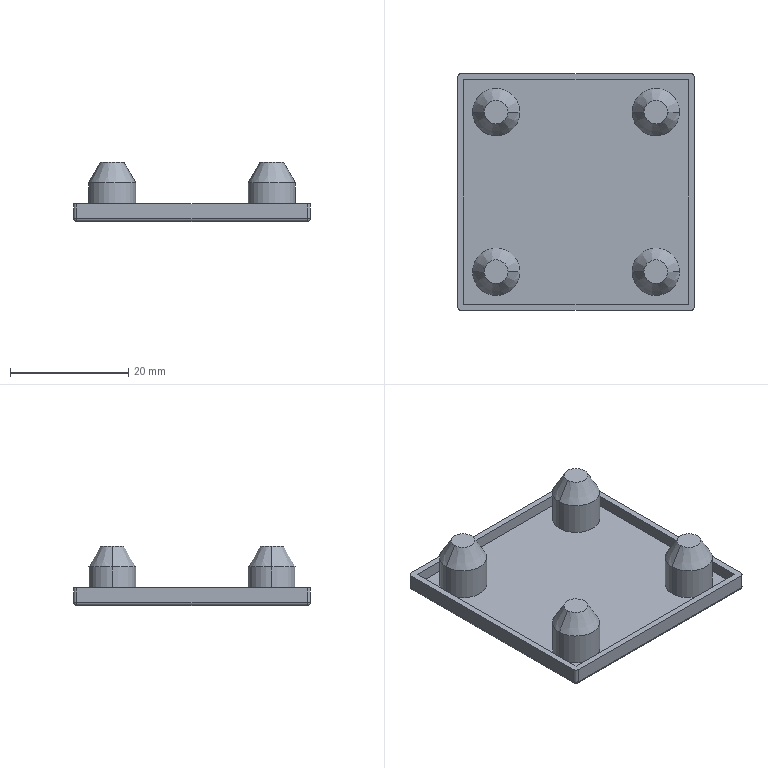Part | NX | 1 solid | 43 faces | box 40 x 40 x 10 mm | volume 3422 mm3 | cylinder 16 | plane 15 | cone 8 | sphere 4 | commonest cylinder face diameters 1 x8 8 x8
STEP:
#1=CARTESIAN_POINT('',(-19.5,19.5,0.));
#2=VERTEX_POINT('',#1);
#3=CARTESIAN_POINT('',(19.5,19.5,0.));
#4=VERTEX_POINT('',#3);
#5=CARTESIAN_POINT('',(-20.1,19.5,0.));
#6=DIRECTION('',(1.,0.,0.));
#7=VECTOR('',#6,1000.);
#8=LINE('',#5,#7);
#9=EDGE_CURVE('',#2,#4,#8,.T.);
#10=ORIENTED_EDGE('',*,*,#9,.T.);
#11=CARTESIAN_POINT('',(19.5,-19.5,0.));
#12=VERTEX_POINT('',#11);
#13=CARTESIAN_POINT('',(19.5,20.097,0.));
#14=DIRECTION('',(0.,-1.,0.));
#15=VECTOR('',#14,1000.);
#16=LINE('',#13,#15);
#17=EDGE_CURVE('',#4,#12,#16,.T.);
#18=ORIENTED_EDGE('',*,*,#17,.T.);
#19=CARTESIAN_POINT('',(-19.5,-19.5,0.));
#20=VERTEX_POINT('',#19);
#21=CARTESIAN_POINT('',(20.092,-19.5,0.));
#22=DIRECTION('',(-1.,0.,0.));
#23=VECTOR('',#22,1000.);
#24=LINE('',#21,#23);
#25=EDGE_CURVE('',#12,#20,#24,.T.);
#26=ORIENTED_EDGE('',*,*,#25,.T.);
#27=CARTESIAN_POINT('',(-19.5,-20.094,0.));
#28=DIRECTION('',(0.,1.,0.));
#29=VECTOR('',#28,1000.);
#30=LINE('',#27,#29);
#31=EDGE_CURVE('',#20,#2,#30,.T.);
#32=ORIENTED_EDGE('',*,*,#31,.T.);
#33=EDGE_LOOP('',(#10,#18,#26,#32));
#34=FACE_BOUND('',#33,.T.);
#35=CARTESIAN_POINT('',(0.,0.,0.));
#36=DIRECTION('',(0.,0.,1.));
#37=DIRECTION('',(1.,0.,0.));
#38=AXIS2_PLACEMENT_3D('',#35,#36,#37);
#39=PLANE('',#38);
#40=ADVANCED_FACE('',(#34),#39,.F.);
#41=CARTESIAN_POINT('',(19.5,20.,0.5));
#42=VERTEX_POINT('',#41);
#43=CARTESIAN_POINT('',(-19.5,20.,0.5));
#44=VERTEX_POINT('',#43);
#45=CARTESIAN_POINT('',(19.5,20.,0.5));
#46=DIRECTION('',(-1.,0.,0.));
#47=VECTOR('',#46,1000.);
#48=LINE('',#45,#47);
#49=EDGE_CURVE('',#42,#44,#48,.T.);
#50=ORIENTED_EDGE('',*,*,#49,.F.);
#51=CARTESIAN_POINT('',(19.5,19.5,0.5));
#52=DIRECTION('',(-1.,0.,0.));
#53=DIRECTION('',(0.,1.,0.));
#54=AXIS2_PLACEMENT_3D('',#51,#52,#53);
#55=CIRCLE('',#54,0.5);
#56=EDGE_CURVE('',#42,#4,#55,.T.);
#57=ORIENTED_EDGE('',*,*,#56,.T.);
#58=ORIENTED_EDGE('',*,*,#9,.F.);
#59=CARTESIAN_POINT('',(-19.5,19.5,0.5));
#60=DIRECTION('',(1.,0.,0.));
#61=DIRECTION('',(0.,0.,-1.));
#62=AXIS2_PLACEMENT_3D('',#59,#60,#61);
#63=CIRCLE('',#62,0.5);
#64=EDGE_CURVE('',#2,#44,#63,.T.);
#65=ORIENTED_EDGE('',*,*,#64,.T.);
#66=EDGE_LOOP('',(#50,#57,#58,#65));
#67=FACE_BOUND('',#66,.T.);
#68=CARTESIAN_POINT('',(-20.1,19.5,0.5));
#69=DIRECTION('',(1.,0.,0.));
#70=DIRECTION('',(0.,0.,-1.));
#71=AXIS2_PLACEMENT_3D('',#68,#69,#70);
#72=CYLINDRICAL_SURFACE('',#71,0.5);
#73=ADVANCED_FACE('',(#67),#72,.T.);
#74=CARTESIAN_POINT('',(19.5,20.,3.));
#75=VERTEX_POINT('',#74);
#76=CARTESIAN_POINT('',(19.5,20.,3.097));
#77=DIRECTION('',(0.,0.,-1.));
#78=VECTOR('',#77,1000.);
#79=LINE('',#76,#78);
#80=EDGE_CURVE('',#75,#42,#79,.T.);
#81=ORIENTED_EDGE('',*,*,#80,.T.);
#82=ORIENTED_EDGE('',*,*,#49,.T.);
#83=CARTESIAN_POINT('',(-19.5,20.,3.));
#84=VERTEX_POINT('',#83);
#85=CARTESIAN_POINT('',(-19.5,20.,0.5));
#86=DIRECTION('',(0.,0.,1.));
#87=VECTOR('',#86,1000.);
#88=LINE('',#85,#87);
#89=EDGE_CURVE('',#44,#84,#88,.T.);
#90=ORIENTED_EDGE('',*,*,#89,.T.);
#91=CARTESIAN_POINT('',(-19.5,20.,3.));
#92=DIRECTION('',(1.,0.,0.));
#93=VECTOR('',#92,1000.);
#94=LINE('',#91,#93);
#95=EDGE_CURVE('',#84,#75,#94,.T.);
#96=ORIENTED_EDGE('',*,*,#95,.T.);
#97=EDGE_LOOP('',(#81,#82,#90,#96));
#98=FACE_BOUND('',#97,.T.);
#99=CARTESIAN_POINT('',(20.,20.,0.));
#100=DIRECTION('',(0.,1.,0.));
#101=DIRECTION('',(1.,0.,0.));
#102=AXIS2_PLACEMENT_3D('',#99,#100,#101);
#103=PLANE('',#102);
#104=ADVANCED_FACE('',(#98),#103,.T.);
#105=ORIENTED_EDGE('',*,*,#80,.F.);
#106=CARTESIAN_POINT('',(20.,19.5,3.));
#107=VERTEX_POINT('',#106);
#108=CARTESIAN_POINT('',(19.5,19.5,3.));
#109=DIRECTION('',(0.,0.,-1.));
#110=DIRECTION('',(0.,1.,0.));
#111=AXIS2_PLACEMENT_3D('',#108,#109,#110);
#112=CIRCLE('',#111,0.5);
#113=EDGE_CURVE('',#75,#107,#112,.T.);
#114=ORIENTED_EDGE('',*,*,#113,.T.);
#115=CARTESIAN_POINT('',(20.,19.5,0.5));
#116=VERTEX_POINT('',#115);
#117=CARTESIAN_POINT('',(20.,19.5,0.5));
#118=DIRECTION('',(0.,0.,1.));
#119=VECTOR('',#118,1000.);
#120=LINE('',#117,#119);
#121=EDGE_CURVE('',#116,#107,#120,.T.);
#122=ORIENTED_EDGE('',*,*,#121,.F.);
#123=CARTESIAN_POINT('',(19.5,19.5,0.5));
#124=DIRECTION('',(0.,0.,1.));
#125=DIRECTION('',(-1.,0.,0.));
#126=AXIS2_PLACEMENT_3D('',#123,#124,#125);
#127=CIRCLE('',#126,0.5);
#128=EDGE_CURVE('',#116,#42,#127,.T.);
#129=ORIENTED_EDGE('',*,*,#128,.T.);
#130=EDGE_LOOP('',(#105,#114,#122,#129));
#131=FACE_BOUND('',#130,.T.);
#132=CARTESIAN_POINT('',(19.5,19.5,3.097));
#133=DIRECTION('',(0.,0.,-1.));
#134=DIRECTION('',(0.,1.,0.));
#135=AXIS2_PLACEMENT_3D('',#132,#133,#134);
#136=CYLINDRICAL_SURFACE('',#135,0.5);
#137=ADVANCED_FACE('',(#131),#136,.T.);
#138=CARTESIAN_POINT('',(19.5,19.5,0.5));
#139=DIRECTION('',(0.,1.,0.));
#140=DIRECTION('',(1.,0.,0.));
#141=AXIS2_PLACEMENT_3D('',#138,#139,#140);
#142=CIRCLE('',#141,0.5);
#143=EDGE_CURVE('',#116,#4,#142,.T.);
#144=ORIENTED_EDGE('',*,*,#143,.T.);
#145=ORIENTED_EDGE('',*,*,#56,.F.);
#146=ORIENTED_EDGE('',*,*,#128,.F.);
#147=EDGE_LOOP('',(#144,#145,#146));
#148=FACE_BOUND('',#147,.T.);
#149=CARTESIAN_POINT('',(19.5,19.5,0.5));
#150=DIRECTION('',(0.,1.,0.));
#151=DIRECTION('',(1.,0.,0.));
#152=AXIS2_PLACEMENT_3D('',#149,#150,#151);
#153=SPHERICAL_SURFACE('',#152,0.5);
#154=ADVANCED_FACE('',(#148),#153,.T.);
#155=ORIENTED_EDGE('',*,*,#17,.F.);
#156=ORIENTED_EDGE('',*,*,#143,.F.);
#157=CARTESIAN_POINT('',(20.,-19.5,0.5));
#158=VERTEX_POINT('',#157);
#159=CARTESIAN_POINT('',(20.,-19.5,0.5));
#160=DIRECTION('',(0.,1.,0.));
#161=VECTOR('',#160,1000.);
#162=LINE('',#159,#161);
#163=EDGE_CURVE('',#158,#116,#162,.T.);
#164=ORIENTED_EDGE('',*,*,#163,.F.);
#165=CARTESIAN_POINT('',(19.5,-19.5,0.5));
#166=DIRECTION('',(0.,1.,0.));
#167=DIRECTION('',(1.,0.,0.));
#168=AXIS2_PLACEMENT_3D('',#165,#166,#167);
#169=CIRCLE('',#168,0.5);
#170=EDGE_CURVE('',#158,#12,#169,.T.);
#171=ORIENTED_EDGE('',*,*,#170,.T.);
#172=EDGE_LOOP('',(#155,#156,#164,#171));
#173=FACE_BOUND('',#172,.T.);
#174=CARTESIAN_POINT('',(19.5,20.097,0.5));
#175=DIRECTION('',(0.,-1.,0.));
#176=DIRECTION('',(0.,0.,-1.));
#177=AXIS2_PLACEMENT_3D('',#174,#175,#176);
#178=CYLINDRICAL_SURFACE('',#177,0.5);
#179=ADVANCED_FACE('',(#173),#178,.T.);
#180=CARTESIAN_POINT('',(19.5,-20.,0.5));
#181=VERTEX_POINT('',#180);
#182=CARTESIAN_POINT('',(19.5,-19.5,0.5));
#183=DIRECTION('',(-1.,0.,0.));
#184=DIRECTION('',(0.,0.,-1.));
#185=AXIS2_PLACEMENT_3D('',#182,#183,#184);
#186=CIRCLE('',#185,0.5);
#187=EDGE_CURVE('',#12,#181,#186,.T.);
#188=ORIENTED_EDGE('',*,*,#187,.F.);
#189=ORIENTED_EDGE('',*,*,#170,.F.);
#190=CARTESIAN_POINT('',(19.5,-19.5,0.5));
#191=DIRECTION('',(0.,0.,1.));
#192=DIRECTION('',(-1.,0.,0.));
#193=AXIS2_PLACEMENT_3D('',#190,#191,#192);
#194=CIRCLE('',#193,0.5);
#195=EDGE_CURVE('',#181,#158,#194,.T.);
#196=ORIENTED_EDGE('',*,*,#195,.F.);
#197=EDGE_LOOP('',(#188,#189,#196));
#198=FACE_BOUND('',#197,.T.);
#199=CARTESIAN_POINT('',(19.5,-19.5,0.5));
#200=DIRECTION('',(0.,1.,0.));
#201=DIRECTION('',(1.,0.,0.));
#202=AXIS2_PLACEMENT_3D('',#199,#200,#201);
#203=SPHERICAL_SURFACE('',#202,0.5);
#204=ADVANCED_FACE('',(#198),#203,.T.);
#205=ORIENTED_EDGE('',*,*,#25,.F.);
#206=ORIENTED_EDGE('',*,*,#187,.T.);
#207=CARTESIAN_POINT('',(-19.5,-20.,0.5));
#208=VERTEX_POINT('',#207);
#209=CARTESIAN_POINT('',(-19.5,-20.,0.5));
#210=DIRECTION('',(1.,0.,0.));
#211=VECTOR('',#210,1000.);
#212=LINE('',#209,#211);
#213=EDGE_CURVE('',#208,#181,#212,.T.);
#214=ORIENTED_EDGE('',*,*,#213,.F.);
#215=CARTESIAN_POINT('',(-19.5,-19.5,0.5));
#216=DIRECTION('',(1.,0.,0.));
#217=DIRECTION('',(0.,-1.,0.));
#218=AXIS2_PLACEMENT_3D('',#215,#216,#217);
#219=CIRCLE('',#218,0.5);
#220=EDGE_CURVE('',#208,#20,#219,.T.);
#221=ORIENTED_EDGE('',*,*,#220,.T.);
#222=EDGE_LOOP('',(#205,#206,#214,#221));
#223=FACE_BOUND('',#222,.T.);
#224=CARTESIAN_POINT('',(20.092,-19.5,0.5));
#225=DIRECTION('',(-1.,0.,0.));
#226=DIRECTION('',(0.,0.,-1.));
#227=AXIS2_PLACEMENT_3D('',#224,#225,#226);
#228=CYLINDRICAL_SURFACE('',#227,0.5);
#229=ADVANCED_FACE('',(#223),#228,.T.);
#230=CARTESIAN_POINT('',(-20.,-19.5,0.5));
#231=VERTEX_POINT('',#230);
#232=CARTESIAN_POINT('',(-19.5,-19.5,0.5));
#233=DIRECTION('',(0.,1.,0.));
#234=DIRECTION('',(1.,0.,0.));
#235=AXIS2_PLACEMENT_3D('',#232,#233,#234);
#236=CIRCLE('',#235,0.5);
#237=EDGE_CURVE('',#20,#231,#236,.T.);
#238=ORIENTED_EDGE('',*,*,#237,.F.);
#239=ORIENTED_EDGE('',*,*,#220,.F.);
#240=CARTESIAN_POINT('',(-19.5,-19.5,0.5));
#241=DIRECTION('',(0.,0.,1.));
#242=DIRECTION('',(-1.,0.,0.));
#243=AXIS2_PLACEMENT_3D('',#240,#241,#242);
#244=CIRCLE('',#243,0.5);
#245=EDGE_CURVE('',#231,#208,#244,.T.);
#246=ORIENTED_EDGE('',*,*,#245,.F.);
#247=EDGE_LOOP('',(#238,#239,#246));
#248=FACE_BOUND('',#247,.T.);
#249=CARTESIAN_POINT('',(-19.5,-19.5,0.5));
#250=DIRECTION('',(0.,1.,0.));
#251=DIRECTION('',(1.,0.,0.));
#252=AXIS2_PLACEMENT_3D('',#249,#250,#251);
#253=SPHERICAL_SURFACE('',#252,0.5);
#254=ADVANCED_FACE('',(#248),#253,.T.);
#255=CARTESIAN_POINT('',(-20.,19.5,0.5));
#256=VERTEX_POINT('',#255);
#257=CARTESIAN_POINT('',(-20.,19.5,0.5));
#258=DIRECTION('',(0.,-1.,0.));
#259=VECTOR('',#258,1000.);
#260=LINE('',#257,#259);
#261=EDGE_CURVE('',#256,#231,#260,.T.);
#262=ORIENTED_EDGE('',*,*,#261,.F.);
#263=CARTESIAN_POINT('',(-19.5,19.5,0.5));
#264=DIRECTION('',(0.,1.,0.));
#265=DIRECTION('',(1.,0.,0.));
#266=AXIS2_PLACEMENT_3D('',#263,#264,#265);
#267=CIRCLE('',#266,0.5);
#268=EDGE_CURVE('',#2,#256,#267,.T.);
#269=ORIENTED_EDGE('',*,*,#268,.F.);
#270=ORIENTED_EDGE('',*,*,#31,.F.);
#271=ORIENTED_EDGE('',*,*,#237,.T.);
#272=EDGE_LOOP('',(#262,#269,#270,#271));
#273=FACE_BOUND('',#272,.T.);
#274=CARTESIAN_POINT('',(-19.5,-20.094,0.5));
#275=DIRECTION('',(0.,1.,0.));
#276=DIRECTION('',(0.,0.,-1.));
#277=AXIS2_PLACEMENT_3D('',#274,#275,#276);
#278=CYLINDRICAL_SURFACE('',#277,0.5);
#279=ADVANCED_FACE('',(#273),#278,.T.);
#280=CARTESIAN_POINT('',(-20.,-19.5,3.));
#281=VERTEX_POINT('',#280);
#282=CARTESIAN_POINT('',(-20.,-19.5,0.5));
#283=DIRECTION('',(0.,0.,1.));
#284=VECTOR('',#283,1000.);
#285=LINE('',#282,#284);
#286=EDGE_CURVE('',#231,#281,#285,.T.);
#287=ORIENTED_EDGE('',*,*,#286,.T.);
#288=CARTESIAN_POINT('',(-20.,19.5,3.));
#289=VERTEX_POINT('',#288);
#290=CARTESIAN_POINT('',(-20.,-19.5,3.));
#291=DIRECTION('',(0.,1.,0.));
#292=VECTOR('',#291,1000.);
#293=LINE('',#290,#292);
#294=EDGE_CURVE('',#281,#289,#293,.T.);
#295=ORIENTED_EDGE('',*,*,#294,.T.);
#296=CARTESIAN_POINT('',(-20.,19.5,3.097));
#297=DIRECTION('',(0.,0.,-1.));
#298=VECTOR('',#297,1000.);
#299=LINE('',#296,#298);
#300=EDGE_CURVE('',#289,#256,#299,.T.);
#301=ORIENTED_EDGE('',*,*,#300,.T.);
#302=ORIENTED_EDGE('',*,*,#261,.T.);
#303=EDGE_LOOP('',(#287,#295,#301,#302));
#304=FACE_BOUND('',#303,.T.);
#305=CARTESIAN_POINT('',(-20.,20.,0.));
#306=DIRECTION('',(-1.,0.,0.));
#307=DIRECTION('',(0.,0.,1.));
#308=AXIS2_PLACEMENT_3D('',#305,#306,#307);
#309=PLANE('',#308);
#310=ADVANCED_FACE('',(#304),#309,.T.);
#311=CARTESIAN_POINT('',(-19.5,-20.,3.));
#312=VERTEX_POINT('',#311);
#313=CARTESIAN_POINT('',(-19.5,-20.,3.097));
#314=DIRECTION('',(0.,0.,-1.));
#315=VECTOR('',#314,1000.);
#316=LINE('',#313,#315);
#317=EDGE_CURVE('',#312,#208,#316,.T.);
#318=ORIENTED_EDGE('',*,*,#317,.F.);
#319=CARTESIAN_POINT('',(-19.5,-19.5,3.));
#320=DIRECTION('',(0.,0.,-1.));
#321=DIRECTION('',(0.,-1.,0.));
#322=AXIS2_PLACEMENT_3D('',#319,#320,#321);
#323=CIRCLE('',#322,0.5);
#324=EDGE_CURVE('',#312,#281,#323,.T.);
#325=ORIENTED_EDGE('',*,*,#324,.T.);
#326=ORIENTED_EDGE('',*,*,#286,.F.);
#327=ORIENTED_EDGE('',*,*,#245,.T.);
#328=EDGE_LOOP('',(#318,#325,#326,#327));
#329=FACE_BOUND('',#328,.T.);
#330=CARTESIAN_POINT('',(-19.5,-19.5,3.097));
#331=DIRECTION('',(0.,0.,-1.));
#332=DIRECTION('',(0.,-1.,0.));
#333=AXIS2_PLACEMENT_3D('',#330,#331,#332);
#334=CYLINDRICAL_SURFACE('',#333,0.5);
#335=ADVANCED_FACE('',(#329),#334,.T.);
#336=ORIENTED_EDGE('',*,*,#317,.T.);
#337=ORIENTED_EDGE('',*,*,#213,.T.);
#338=CARTESIAN_POINT('',(19.5,-20.,3.));
#339=VERTEX_POINT('',#338);
#340=CARTESIAN_POINT('',(19.5,-20.,0.5));
#341=DIRECTION('',(0.,0.,1.));
#342=VECTOR('',#341,1000.);
#343=LINE('',#340,#342);
#344=EDGE_CURVE('',#181,#339,#343,.T.);
#345=ORIENTED_EDGE('',*,*,#344,.T.);
#346=CARTESIAN_POINT('',(19.5,-20.,3.));
#347=DIRECTION('',(-1.,0.,0.));
#348=VECTOR('',#347,1000.);
#349=LINE('',#346,#348);
#350=EDGE_CURVE('',#339,#312,#349,.T.);
#351=ORIENTED_EDGE('',*,*,#350,.T.);
#352=EDGE_LOOP('',(#336,#337,#345,#351));
#353=FACE_BOUND('',#352,.T.);
#354=CARTESIAN_POINT('',(-20.,-20.,0.));
#355=DIRECTION('',(0.,-1.,0.));
#356=DIRECTION('',(0.,0.,-1.));
#357=AXIS2_PLACEMENT_3D('',#354,#355,#356);
#358=PLANE('',#357);
#359=ADVANCED_FACE('',(#353),#358,.T.);
#360=ORIENTED_EDGE('',*,*,#324,.F.);
#361=ORIENTED_EDGE('',*,*,#350,.F.);
#362=CARTESIAN_POINT('',(20.,-19.5,3.));
#363=VERTEX_POINT('',#362);
#364=CARTESIAN_POINT('',(19.5,-19.5,3.));
#365=DIRECTION('',(0.,0.,-1.));
#366=DIRECTION('',(1.,0.,0.));
#367=AXIS2_PLACEMENT_3D('',#364,#365,#366);
#368=CIRCLE('',#367,0.5);
#369=EDGE_CURVE('',#363,#339,#368,.T.);
#370=ORIENTED_EDGE('',*,*,#369,.F.);
#371=CARTESIAN_POINT('',(20.,19.5,3.));
#372=DIRECTION('',(0.,-1.,0.));
#373=VECTOR('',#372,1000.);
#374=LINE('',#371,#373);
#375=EDGE_CURVE('',#107,#363,#374,.T.);
#376=ORIENTED_EDGE('',*,*,#375,.F.);
#377=ORIENTED_EDGE('',*,*,#113,.F.);
#378=ORIENTED_EDGE('',*,*,#95,.F.);
#379=CARTESIAN_POINT('',(-19.5,19.5,3.));
#380=DIRECTION('',(0.,0.,-1.));
#381=DIRECTION('',(-1.,0.,0.));
#382=AXIS2_PLACEMENT_3D('',#379,#380,#381);
#383=CIRCLE('',#382,0.5);
#384=EDGE_CURVE('',#289,#84,#383,.T.);
#385=ORIENTED_EDGE('',*,*,#384,.F.);
#386=ORIENTED_EDGE('',*,*,#294,.F.);
#387=EDGE_LOOP('',(#360,#361,#370,#376,#377,#378,#385,#386));
#388=FACE_BOUND('',#387,.T.);
#389=CARTESIAN_POINT('',(-19.,-19.,3.));
#390=VERTEX_POINT('',#389);
#391=CARTESIAN_POINT('',(-19.,19.,3.));
#392=VERTEX_POINT('',#391);
#393=CARTESIAN_POINT('',(-19.,-19.,3.));
#394=DIRECTION('',(0.,1.,0.));
#395=VECTOR('',#394,1000.);
#396=LINE('',#393,#395);
#397=EDGE_CURVE('',#390,#392,#396,.T.);
#398=ORIENTED_EDGE('',*,*,#397,.T.);
#399=CARTESIAN_POINT('',(19.,19.,3.));
#400=VERTEX_POINT('',#399);
#401=CARTESIAN_POINT('',(-19.,19.,3.));
#402=DIRECTION('',(1.,0.,0.));
#403=VECTOR('',#402,1000.);
#404=LINE('',#401,#403);
#405=EDGE_CURVE('',#392,#400,#404,.T.);
#406=ORIENTED_EDGE('',*,*,#405,.T.);
#407=CARTESIAN_POINT('',(19.,-19.,3.));
#408=VERTEX_POINT('',#407);
#409=CARTESIAN_POINT('',(19.,19.,3.));
#410=DIRECTION('',(0.,-1.,0.));
#411=VECTOR('',#410,1000.);
#412=LINE('',#409,#411);
#413=EDGE_CURVE('',#400,#408,#412,.T.);
#414=ORIENTED_EDGE('',*,*,#413,.T.);
#415=CARTESIAN_POINT('',(19.,-19.,3.));
#416=DIRECTION('',(-1.,0.,0.));
#417=VECTOR('',#416,1000.);
#418=LINE('',#415,#417);
#419=EDGE_CURVE('',#408,#390,#418,.T.);
#420=ORIENTED_EDGE('',*,*,#419,.T.);
#421=EDGE_LOOP('',(#398,#406,#414,#420));
#422=FACE_BOUND('',#421,.T.);
#423=CARTESIAN_POINT('',(0.,0.,3.));
#424=DIRECTION('',(0.,0.,1.));
#425=DIRECTION('',(1.,0.,0.));
#426=AXIS2_PLACEMENT_3D('',#423,#424,#425);
#427=PLANE('',#426);
#428=ADVANCED_FACE('',(#388,#422),#427,.T.);
#429=ORIENTED_EDGE('',*,*,#300,.F.);
#430=ORIENTED_EDGE('',*,*,#384,.T.);
#431=ORIENTED_EDGE('',*,*,#89,.F.);
#432=CARTESIAN_POINT('',(-19.5,19.5,0.5));
#433=DIRECTION('',(0.,0.,1.));
#434=DIRECTION('',(-1.,0.,0.));
#435=AXIS2_PLACEMENT_3D('',#432,#433,#434);
#436=CIRCLE('',#435,0.5);
#437=EDGE_CURVE('',#44,#256,#436,.T.);
#438=ORIENTED_EDGE('',*,*,#437,.T.);
#439=EDGE_LOOP('',(#429,#430,#431,#438));
#440=FACE_BOUND('',#439,.T.);
#441=CARTESIAN_POINT('',(-19.5,19.5,3.097));
#442=DIRECTION('',(0.,0.,-1.));
#443=DIRECTION('',(-1.,0.,0.));
#444=AXIS2_PLACEMENT_3D('',#441,#442,#443);
#445=CYLINDRICAL_SURFACE('',#444,0.5);
#446=ADVANCED_FACE('',(#440),#445,.T.);
#447=ORIENTED_EDGE('',*,*,#268,.T.);
#448=ORIENTED_EDGE('',*,*,#437,.F.);
#449=ORIENTED_EDGE('',*,*,#64,.F.);
#450=EDGE_LOOP('',(#447,#448,#449));
#451=FACE_BOUND('',#450,.T.);
#452=CARTESIAN_POINT('',(-19.5,19.5,0.5));
#453=DIRECTION('',(0.,1.,0.));
#454=DIRECTION('',(1.,0.,0.));
#455=AXIS2_PLACEMENT_3D('',#452,#453,#454);
#456=SPHERICAL_SURFACE('',#455,0.5);
#457=ADVANCED_FACE('',(#451),#456,.T.);
#458=CARTESIAN_POINT('',(20.,-19.5,3.097));
#459=DIRECTION('',(0.,0.,-1.));
#460=VECTOR('',#459,1000.);
#461=LINE('',#458,#460);
#462=EDGE_CURVE('',#363,#158,#461,.T.);
#463=ORIENTED_EDGE('',*,*,#462,.T.);
#464=ORIENTED_EDGE('',*,*,#163,.T.);
#465=ORIENTED_EDGE('',*,*,#121,.T.);
#466=ORIENTED_EDGE('',*,*,#375,.T.);
#467=EDGE_LOOP('',(#463,#464,#465,#466));
#468=FACE_BOUND('',#467,.T.);
#469=CARTESIAN_POINT('',(20.,-20.,0.));
#470=DIRECTION('',(1.,0.,0.));
#471=DIRECTION('',(0.,1.,0.));
#472=AXIS2_PLACEMENT_3D('',#469,#470,#471);
#473=PLANE('',#472);
#474=ADVANCED_FACE('',(#468),#473,.T.);
#475=ORIENTED_EDGE('',*,*,#462,.F.);
#476=ORIENTED_EDGE('',*,*,#369,.T.);
#477=ORIENTED_EDGE('',*,*,#344,.F.);
#478=ORIENTED_EDGE('',*,*,#195,.T.);
#479=EDGE_LOOP('',(#475,#476,#477,#478));
#480=FACE_BOUND('',#479,.T.);
#481=CARTESIAN_POINT('',(19.5,-19.5,3.097));
#482=DIRECTION('',(0.,0.,-1.));
#483=DIRECTION('',(1.,0.,0.));
#484=AXIS2_PLACEMENT_3D('',#481,#482,#483);
#485=CYLINDRICAL_SURFACE('',#484,0.5);
#486=ADVANCED_FACE('',(#480),#485,.T.);
#487=ORIENTED_EDGE('',*,*,#397,.F.);
#488=CARTESIAN_POINT('',(-19.,-19.,1.));
#489=VERTEX_POINT('',#488);
#490=CARTESIAN_POINT('',(-19.,-19.,3.));
#491=DIRECTION('',(0.,0.,-1.));
#492=VECTOR('',#491,1000.);
#493=LINE('',#490,#492);
#494=EDGE_CURVE('',#390,#489,#493,.T.);
#495=ORIENTED_EDGE('',*,*,#494,.T.);
#496=CARTESIAN_POINT('',(-19.,19.,1.));
#497=VERTEX_POINT('',#496);
#498=CARTESIAN_POINT('',(-19.,-19.,1.));
#499=DIRECTION('',(0.,1.,0.));
#500=VECTOR('',#499,1000.);
#501=LINE('',#498,#500);
#502=EDGE_CURVE('',#489,#497,#501,.T.);
#503=ORIENTED_EDGE('',*,*,#502,.T.);
#504=CARTESIAN_POINT('',(-19.,19.,3.));
#505=DIRECTION('',(0.,0.,-1.));
#506=VECTOR('',#505,1000.);
#507=LINE('',#504,#506);
#508=EDGE_CURVE('',#392,#497,#507,.T.);
#509=ORIENTED_EDGE('',*,*,#508,.F.);
#510=EDGE_LOOP('',(#487,#495,#503,#509));
#511=FACE_BOUND('',#510,.T.);
#512=CARTESIAN_POINT('',(-19.,20.,0.));
#513=DIRECTION('',(-1.,0.,0.));
#514=DIRECTION('',(0.,0.,1.));
#515=AXIS2_PLACEMENT_3D('',#512,#513,#514);
#516=PLANE('',#515);
#517=ADVANCED_FACE('',(#511),#516,.F.);
#518=ORIENTED_EDGE('',*,*,#405,.F.);
#519=ORIENTED_EDGE('',*,*,#508,.T.);
#520=CARTESIAN_POINT('',(19.,19.,1.));
#521=VERTEX_POINT('',#520);
#522=CARTESIAN_POINT('',(-19.,19.,1.));
#523=DIRECTION('',(1.,0.,0.));
#524=VECTOR('',#523,1000.);
#525=LINE('',#522,#524);
#526=EDGE_CURVE('',#497,#521,#525,.T.);
#527=ORIENTED_EDGE('',*,*,#526,.T.);
#528=CARTESIAN_POINT('',(19.,19.,3.));
#529=DIRECTION('',(0.,0.,-1.));
#530=VECTOR('',#529,1000.);
#531=LINE('',#528,#530);
#532=EDGE_CURVE('',#400,#521,#531,.T.);
#533=ORIENTED_EDGE('',*,*,#532,.F.);
#534=EDGE_LOOP('',(#518,#519,#527,#533));
#535=FACE_BOUND('',#534,.T.);
#536=CARTESIAN_POINT('',(20.,19.,0.));
#537=DIRECTION('',(0.,1.,0.));
#538=DIRECTION('',(1.,0.,0.));
#539=AXIS2_PLACEMENT_3D('',#536,#537,#538);
#540=PLANE('',#539);
#541=ADVANCED_FACE('',(#535),#540,.F.);
#542=ORIENTED_EDGE('',*,*,#413,.F.);
#543=ORIENTED_EDGE('',*,*,#532,.T.);
#544=CARTESIAN_POINT('',(19.,-19.,1.));
#545=VERTEX_POINT('',#544);
#546=CARTESIAN_POINT('',(19.,19.,1.));
#547=DIRECTION('',(0.,-1.,0.));
#548=VECTOR('',#547,1000.);
#549=LINE('',#546,#548);
#550=EDGE_CURVE('',#521,#545,#549,.T.);
#551=ORIENTED_EDGE('',*,*,#550,.T.);
#552=CARTESIAN_POINT('',(19.,-19.,3.));
#553=DIRECTION('',(0.,0.,-1.));
#554=VECTOR('',#553,1000.);
#555=LINE('',#552,#554);
#556=EDGE_CURVE('',#408,#545,#555,.T.);
#557=ORIENTED_EDGE('',*,*,#556,.F.);
#558=EDGE_LOOP('',(#542,#543,#551,#557));
#559=FACE_BOUND('',#558,.T.);
#560=CARTESIAN_POINT('',(19.,-20.,0.));
#561=DIRECTION('',(1.,0.,0.));
#562=DIRECTION('',(0.,1.,0.));
#563=AXIS2_PLACEMENT_3D('',#560,#561,#562);
#564=PLANE('',#563);
#565=ADVANCED_FACE('',(#559),#564,.F.);
#566=ORIENTED_EDGE('',*,*,#419,.F.);
#567=ORIENTED_EDGE('',*,*,#556,.T.);
#568=CARTESIAN_POINT('',(19.,-19.,1.));
#569=DIRECTION('',(-1.,0.,0.));
#570=VECTOR('',#569,1000.);
#571=LINE('',#568,#570);
#572=EDGE_CURVE('',#545,#489,#571,.T.);
#573=ORIENTED_EDGE('',*,*,#572,.T.);
#574=ORIENTED_EDGE('',*,*,#494,.F.);
#575=EDGE_LOOP('',(#566,#567,#573,#574));
#576=FACE_BOUND('',#575,.T.);
#577=CARTESIAN_POINT('',(-20.,-19.,0.));
#578=DIRECTION('',(0.,-1.,0.));
#579=DIRECTION('',(0.,0.,-1.));
#580=AXIS2_PLACEMENT_3D('',#577,#578,#579);
#581=PLANE('',#580);
#582=ADVANCED_FACE('',(#576),#581,.F.);
#583=ORIENTED_EDGE('',*,*,#502,.F.);
#584=ORIENTED_EDGE('',*,*,#572,.F.);
#585=ORIENTED_EDGE('',*,*,#550,.F.);
#586=ORIENTED_EDGE('',*,*,#526,.F.);
#587=EDGE_LOOP('',(#583,#584,#585,#586));
#588=FACE_BOUND('',#587,.T.);
#589=CARTESIAN_POINT('',(9.5,13.5,1.));
#590=VERTEX_POINT('',#589);
#591=CARTESIAN_POINT('',(17.5,13.5,1.));
#592=VERTEX_POINT('',#591);
#593=CARTESIAN_POINT('',(13.5,13.5,1.));
#594=DIRECTION('',(0.,0.,1.));
#595=DIRECTION('',(-1.,0.,0.));
#596=AXIS2_PLACEMENT_3D('',#593,#594,#595);
#597=CIRCLE('',#596,4.);
#598=EDGE_CURVE('',#590,#592,#597,.T.);
#599=ORIENTED_EDGE('',*,*,#598,.F.);
#600=CARTESIAN_POINT('',(13.5,13.5,1.));
#601=DIRECTION('',(0.,0.,1.));
#602=DIRECTION('',(-1.,0.,0.));
#603=AXIS2_PLACEMENT_3D('',#600,#601,#602);
#604=CIRCLE('',#603,4.);
#605=EDGE_CURVE('',#592,#590,#604,.T.);
#606=ORIENTED_EDGE('',*,*,#605,.F.);
#607=EDGE_LOOP('',(#599,#606));
#608=FACE_BOUND('',#607,.T.);
#609=CARTESIAN_POINT('',(-9.5,13.5,1.));
#610=VERTEX_POINT('',#609);
#611=CARTESIAN_POINT('',(-17.5,13.5,1.));
#612=VERTEX_POINT('',#611);
#613=CARTESIAN_POINT('',(-13.5,13.5,1.));
#614=DIRECTION('',(0.,0.,1.));
#615=DIRECTION('',(-1.,0.,0.));
#616=AXIS2_PLACEMENT_3D('',#613,#614,#615);
#617=CIRCLE('',#616,4.);
#618=EDGE_CURVE('',#610,#612,#617,.T.);
#619=ORIENTED_EDGE('',*,*,#618,.F.);
#620=CARTESIAN_POINT('',(-13.5,13.5,1.));
#621=DIRECTION('',(0.,0.,1.));
#622=DIRECTION('',(-1.,0.,0.));
#623=AXIS2_PLACEMENT_3D('',#620,#621,#622);
#624=CIRCLE('',#623,4.);
#625=EDGE_CURVE('',#612,#610,#624,.T.);
#626=ORIENTED_EDGE('',*,*,#625,.F.);
#627=EDGE_LOOP('',(#619,#626));
#628=FACE_BOUND('',#627,.T.);
#629=CARTESIAN_POINT('',(-17.5,-13.5,1.));
#630=VERTEX_POINT('',#629);
#631=CARTESIAN_POINT('',(-9.5,-13.5,1.));
#632=VERTEX_POINT('',#631);
#633=CARTESIAN_POINT('',(-13.5,-13.5,1.));
#634=DIRECTION('',(0.,0.,1.));
#635=DIRECTION('',(-1.,0.,0.));
#636=AXIS2_PLACEMENT_3D('',#633,#634,#635);
#637=CIRCLE('',#636,4.);
#638=EDGE_CURVE('',#630,#632,#637,.T.);
#639=ORIENTED_EDGE('',*,*,#638,.F.);
#640=CARTESIAN_POINT('',(-13.5,-13.5,1.));
#641=DIRECTION('',(0.,0.,1.));
#642=DIRECTION('',(-1.,0.,0.));
#643=AXIS2_PLACEMENT_3D('',#640,#641,#642);
#644=CIRCLE('',#643,4.);
#645=EDGE_CURVE('',#632,#630,#644,.T.);
#646=ORIENTED_EDGE('',*,*,#645,.F.);
#647=EDGE_LOOP('',(#639,#646));
#648=FACE_BOUND('',#647,.T.);
#649=CARTESIAN_POINT('',(9.5,-13.5,1.));
#650=VERTEX_POINT('',#649);
#651=CARTESIAN_POINT('',(17.5,-13.5,1.));
#652=VERTEX_POINT('',#651);
#653=CARTESIAN_POINT('',(13.5,-13.5,1.));
#654=DIRECTION('',(0.,0.,1.));
#655=DIRECTION('',(-1.,0.,0.));
#656=AXIS2_PLACEMENT_3D('',#653,#654,#655);
#657=CIRCLE('',#656,4.);
#658=EDGE_CURVE('',#650,#652,#657,.T.);
#659=ORIENTED_EDGE('',*,*,#658,.F.);
#660=CARTESIAN_POINT('',(13.5,-13.5,1.));
#661=DIRECTION('',(0.,0.,1.));
#662=DIRECTION('',(-1.,0.,0.));
#663=AXIS2_PLACEMENT_3D('',#660,#661,#662);
#664=CIRCLE('',#663,4.);
#665=EDGE_CURVE('',#652,#650,#664,.T.);
#666=ORIENTED_EDGE('',*,*,#665,.F.);
#667=EDGE_LOOP('',(#659,#666));
#668=FACE_BOUND('',#667,.T.);
#669=CARTESIAN_POINT('',(0.,0.,1.));
#670=DIRECTION('',(0.,0.,1.));
#671=DIRECTION('',(1.,0.,0.));
#672=AXIS2_PLACEMENT_3D('',#669,#670,#671);
#673=PLANE('',#672);
#674=ADVANCED_FACE('',(#588,#608,#628,#648,#668),#673,.T.);
#675=ORIENTED_EDGE('',*,*,#598,.T.);
#676=CARTESIAN_POINT('',(17.5,13.5,6.536));
#677=VERTEX_POINT('',#676);
#678=CARTESIAN_POINT('',(17.5,13.5,0.));
#679=DIRECTION('',(0.,0.,1.));
#680=VECTOR('',#679,1000.);
#681=LINE('',#678,#680);
#682=EDGE_CURVE('',#592,#677,#681,.T.);
#683=ORIENTED_EDGE('',*,*,#682,.T.);
#684=CARTESIAN_POINT('',(9.5,13.5,6.536));
#685=VERTEX_POINT('',#684);
#686=CARTESIAN_POINT('',(13.5,13.5,6.536));
#687=DIRECTION('',(0.,0.,-1.));
#688=DIRECTION('',(1.,0.,0.));
#689=AXIS2_PLACEMENT_3D('',#686,#687,#688);
#690=CIRCLE('',#689,4.);
#691=EDGE_CURVE('',#677,#685,#690,.T.);
#692=ORIENTED_EDGE('',*,*,#691,.T.);
#693=CARTESIAN_POINT('',(9.5,13.5,0.));
#694=DIRECTION('',(0.,0.,1.));
#695=VECTOR('',#694,1000.);
#696=LINE('',#693,#695);
#697=EDGE_CURVE('',#590,#685,#696,.T.);
#698=ORIENTED_EDGE('',*,*,#697,.F.);
#699=EDGE_LOOP('',(#675,#683,#692,#698));
#700=FACE_BOUND('',#699,.T.);
#701=CARTESIAN_POINT('',(13.5,13.5,0.));
#702=DIRECTION('',(0.,0.,1.));
#703=DIRECTION('',(1.,0.,0.));
#704=AXIS2_PLACEMENT_3D('',#701,#702,#703);
#705=CYLINDRICAL_SURFACE('',#704,4.);
#706=ADVANCED_FACE('',(#700),#705,.T.);
#707=ORIENTED_EDGE('',*,*,#658,.T.);
#708=CARTESIAN_POINT('',(17.5,-13.5,6.536));
#709=VERTEX_POINT('',#708);
#710=CARTESIAN_POINT('',(17.5,-13.5,0.));
#711=DIRECTION('',(0.,0.,1.));
#712=VECTOR('',#711,1000.);
#713=LINE('',#710,#712);
#714=EDGE_CURVE('',#652,#709,#713,.T.);
#715=ORIENTED_EDGE('',*,*,#714,.T.);
#716=CARTESIAN_POINT('',(9.5,-13.5,6.536));
#717=VERTEX_POINT('',#716);
#718=CARTESIAN_POINT('',(13.5,-13.5,6.536));
#719=DIRECTION('',(0.,0.,-1.));
#720=DIRECTION('',(1.,0.,0.));
#721=AXIS2_PLACEMENT_3D('',#718,#719,#720);
#722=CIRCLE('',#721,4.);
#723=EDGE_CURVE('',#709,#717,#722,.T.);
#724=ORIENTED_EDGE('',*,*,#723,.T.);
#725=CARTESIAN_POINT('',(9.5,-13.5,0.));
#726=DIRECTION('',(0.,0.,1.));
#727=VECTOR('',#726,1000.);
#728=LINE('',#725,#727);
#729=EDGE_CURVE('',#650,#717,#728,.T.);
#730=ORIENTED_EDGE('',*,*,#729,.F.);
#731=EDGE_LOOP('',(#707,#715,#724,#730));
#732=FACE_BOUND('',#731,.T.);
#733=CARTESIAN_POINT('',(13.5,-13.5,0.));
#734=DIRECTION('',(0.,0.,1.));
#735=DIRECTION('',(1.,0.,0.));
#736=AXIS2_PLACEMENT_3D('',#733,#734,#735);
#737=CYLINDRICAL_SURFACE('',#736,4.);
#738=ADVANCED_FACE('',(#732),#737,.T.);
#739=ORIENTED_EDGE('',*,*,#691,.F.);
#740=CARTESIAN_POINT('',(15.5,13.5,10.));
#741=VERTEX_POINT('',#740);
#742=CARTESIAN_POINT('',(16.5,13.5,8.268));
#743=DIRECTION('',(0.5,0.,-0.866));
#744=VECTOR('',#743,1000.);
#745=LINE('',#742,#744);
#746=EDGE_CURVE('',#677,#741,#745,.F.);
#747=ORIENTED_EDGE('',*,*,#746,.T.);
#748=CARTESIAN_POINT('',(11.5,13.5,10.));
#749=VERTEX_POINT('',#748);
#750=CARTESIAN_POINT('',(13.5,13.5,10.));
#751=DIRECTION('',(0.,0.,-1.));
#752=DIRECTION('',(-1.,0.,0.));
#753=AXIS2_PLACEMENT_3D('',#750,#751,#752);
#754=CIRCLE('',#753,2.);
#755=EDGE_CURVE('',#741,#749,#754,.T.);
#756=ORIENTED_EDGE('',*,*,#755,.T.);
#757=CARTESIAN_POINT('',(10.5,13.5,8.268));
#758=DIRECTION('',(-0.5,0.,-0.866));
#759=VECTOR('',#758,1000.);
#760=LINE('',#757,#759);
#761=EDGE_CURVE('',#685,#749,#760,.F.);
#762=ORIENTED_EDGE('',*,*,#761,.F.);
#763=EDGE_LOOP('',(#739,#747,#756,#762));
#764=FACE_BOUND('',#763,.T.);
#765=CARTESIAN_POINT('',(13.5,13.5,8.268));
#766=DIRECTION('',(0.,0.,-1.));
#767=DIRECTION('',(-1.,0.,0.));
#768=AXIS2_PLACEMENT_3D('',#765,#766,#767);
#769=CONICAL_SURFACE('',#768,3.,0.5236);
#770=ADVANCED_FACE('',(#764),#769,.T.);
#771=ORIENTED_EDGE('',*,*,#755,.F.);
#772=CARTESIAN_POINT('',(13.5,13.5,10.));
#773=DIRECTION('',(0.,0.,-1.));
#774=DIRECTION('',(-1.,0.,0.));
#775=AXIS2_PLACEMENT_3D('',#772,#773,#774);
#776=CIRCLE('',#775,2.);
#777=EDGE_CURVE('',#749,#741,#776,.T.);
#778=ORIENTED_EDGE('',*,*,#777,.F.);
#779=EDGE_LOOP('',(#771,#778));
#780=FACE_BOUND('',#779,.T.);
#781=CARTESIAN_POINT('',(0.,0.,10.));
#782=DIRECTION('',(0.,0.,1.));
#783=DIRECTION('',(1.,0.,0.));
#784=AXIS2_PLACEMENT_3D('',#781,#782,#783);
#785=PLANE('',#784);
#786=ADVANCED_FACE('',(#780),#785,.T.);
#787=CARTESIAN_POINT('',(11.5,-13.5,10.));
#788=VERTEX_POINT('',#787);
#789=CARTESIAN_POINT('',(15.5,-13.5,10.));
#790=VERTEX_POINT('',#789);
#791=CARTESIAN_POINT('',(13.5,-13.5,10.));
#792=DIRECTION('',(0.,0.,-1.));
#793=DIRECTION('',(-1.,0.,0.));
#794=AXIS2_PLACEMENT_3D('',#791,#792,#793);
#795=CIRCLE('',#794,2.);
#796=EDGE_CURVE('',#788,#790,#795,.T.);
#797=ORIENTED_EDGE('',*,*,#796,.F.);
#798=CARTESIAN_POINT('',(13.5,-13.5,10.));
#799=DIRECTION('',(0.,0.,-1.));
#800=DIRECTION('',(-1.,0.,0.));
#801=AXIS2_PLACEMENT_3D('',#798,#799,#800);
#802=CIRCLE('',#801,2.);
#803=EDGE_CURVE('',#790,#788,#802,.T.);
#804=ORIENTED_EDGE('',*,*,#803,.F.);
#805=EDGE_LOOP('',(#797,#804));
#806=FACE_BOUND('',#805,.T.);
#807=CARTESIAN_POINT('',(0.,0.,10.));
#808=DIRECTION('',(0.,0.,1.));
#809=DIRECTION('',(1.,0.,0.));
#810=AXIS2_PLACEMENT_3D('',#807,#808,#809);
#811=PLANE('',#810);
#812=ADVANCED_FACE('',(#806),#811,.T.);
#813=ORIENTED_EDGE('',*,*,#618,.T.);
#814=CARTESIAN_POINT('',(-17.5,13.5,6.536));
#815=VERTEX_POINT('',#814);
#816=CARTESIAN_POINT('',(-17.5,13.5,0.));
#817=DIRECTION('',(0.,0.,1.));
#818=VECTOR('',#817,1000.);
#819=LINE('',#816,#818);
#820=EDGE_CURVE('',#815,#612,#819,.F.);
#821=ORIENTED_EDGE('',*,*,#820,.F.);
#822=CARTESIAN_POINT('',(-9.5,13.5,6.536));
#823=VERTEX_POINT('',#822);
#824=CARTESIAN_POINT('',(-13.5,13.5,6.536));
#825=DIRECTION('',(0.,0.,-1.));
#826=DIRECTION('',(-1.,0.,0.));
#827=AXIS2_PLACEMENT_3D('',#824,#825,#826);
#828=CIRCLE('',#827,4.);
#829=EDGE_CURVE('',#815,#823,#828,.T.);
#830=ORIENTED_EDGE('',*,*,#829,.T.);
#831=CARTESIAN_POINT('',(-9.5,13.5,0.));
#832=DIRECTION('',(0.,0.,1.));
#833=VECTOR('',#832,1000.);
#834=LINE('',#831,#833);
#835=EDGE_CURVE('',#823,#610,#834,.F.);
#836=ORIENTED_EDGE('',*,*,#835,.T.);
#837=EDGE_LOOP('',(#813,#821,#830,#836));
#838=FACE_BOUND('',#837,.T.);
#839=CARTESIAN_POINT('',(-13.5,13.5,0.));
#840=DIRECTION('',(0.,0.,1.));
#841=DIRECTION('',(1.,0.,0.));
#842=AXIS2_PLACEMENT_3D('',#839,#840,#841);
#843=CYLINDRICAL_SURFACE('',#842,4.);
#844=ADVANCED_FACE('',(#838),#843,.T.);
#845=CARTESIAN_POINT('',(-17.5,-13.5,6.536));
#846=VERTEX_POINT('',#845);
#847=CARTESIAN_POINT('',(-9.5,-13.5,6.536));
#848=VERTEX_POINT('',#847);
#849=CARTESIAN_POINT('',(-13.5,-13.5,6.536));
#850=DIRECTION('',(0.,0.,-1.));
#851=DIRECTION('',(-1.,0.,0.));
#852=AXIS2_PLACEMENT_3D('',#849,#850,#851);
#853=CIRCLE('',#852,4.);
#854=EDGE_CURVE('',#846,#848,#853,.T.);
#855=ORIENTED_EDGE('',*,*,#854,.F.);
#856=CARTESIAN_POINT('',(-15.5,-13.5,10.));
#857=VERTEX_POINT('',#856);
#858=CARTESIAN_POINT('',(-16.5,-13.5,8.268));
#859=DIRECTION('',(-0.5,0.,-0.866));
#860=VECTOR('',#859,1000.);
#861=LINE('',#858,#860);
#862=EDGE_CURVE('',#846,#857,#861,.F.);
#863=ORIENTED_EDGE('',*,*,#862,.T.);
#864=CARTESIAN_POINT('',(-11.5,-13.5,10.));
#865=VERTEX_POINT('',#864);
#866=CARTESIAN_POINT('',(-13.5,-13.5,10.));
#867=DIRECTION('',(0.,0.,-1.));
#868=DIRECTION('',(-1.,0.,0.));
#869=AXIS2_PLACEMENT_3D('',#866,#867,#868);
#870=CIRCLE('',#869,2.);
#871=EDGE_CURVE('',#857,#865,#870,.T.);
#872=ORIENTED_EDGE('',*,*,#871,.T.);
#873=CARTESIAN_POINT('',(-10.5,-13.5,8.268));
#874=DIRECTION('',(0.5,0.,-0.866));
#875=VECTOR('',#874,1000.);
#876=LINE('',#873,#875);
#877=EDGE_CURVE('',#848,#865,#876,.F.);
#878=ORIENTED_EDGE('',*,*,#877,.F.);
#879=EDGE_LOOP('',(#855,#863,#872,#878));
#880=FACE_BOUND('',#879,.T.);
#881=CARTESIAN_POINT('',(-13.5,-13.5,8.268));
#882=DIRECTION('',(0.,0.,-1.));
#883=DIRECTION('',(-1.,0.,0.));
#884=AXIS2_PLACEMENT_3D('',#881,#882,#883);
#885=CONICAL_SURFACE('',#884,3.,0.5236);
#886=ADVANCED_FACE('',(#880),#885,.T.);
#887=CARTESIAN_POINT('',(-13.5,13.5,6.536));
#888=DIRECTION('',(0.,0.,-1.));
#889=DIRECTION('',(-1.,0.,0.));
#890=AXIS2_PLACEMENT_3D('',#887,#888,#889);
#891=CIRCLE('',#890,4.);
#892=EDGE_CURVE('',#823,#815,#891,.T.);
#893=ORIENTED_EDGE('',*,*,#892,.F.);
#894=CARTESIAN_POINT('',(-11.5,13.5,10.));
#895=VERTEX_POINT('',#894);
#896=CARTESIAN_POINT('',(-10.5,13.5,8.268));
#897=DIRECTION('',(0.5,0.,-0.866));
#898=VECTOR('',#897,1000.);
#899=LINE('',#896,#898);
#900=EDGE_CURVE('',#895,#823,#899,.T.);
#901=ORIENTED_EDGE('',*,*,#900,.F.);
#902=CARTESIAN_POINT('',(-15.5,13.5,10.));
#903=VERTEX_POINT('',#902);
#904=CARTESIAN_POINT('',(-13.5,13.5,10.));
#905=DIRECTION('',(0.,0.,-1.));
#906=DIRECTION('',(-1.,0.,0.));
#907=AXIS2_PLACEMENT_3D('',#904,#905,#906);
#908=CIRCLE('',#907,2.);
#909=EDGE_CURVE('',#895,#903,#908,.T.);
#910=ORIENTED_EDGE('',*,*,#909,.T.);
#911=CARTESIAN_POINT('',(-16.5,13.5,8.268));
#912=DIRECTION('',(-0.5,0.,-0.866));
#913=VECTOR('',#912,1000.);
#914=LINE('',#911,#913);
#915=EDGE_CURVE('',#903,#815,#914,.T.);
#916=ORIENTED_EDGE('',*,*,#915,.T.);
#917=EDGE_LOOP('',(#893,#901,#910,#916));
#918=FACE_BOUND('',#917,.T.);
#919=CARTESIAN_POINT('',(-13.5,13.5,8.268));
#920=DIRECTION('',(0.,0.,-1.));
#921=DIRECTION('',(-1.,0.,0.));
#922=AXIS2_PLACEMENT_3D('',#919,#920,#921);
#923=CONICAL_SURFACE('',#922,3.,0.5236);
#924=ADVANCED_FACE('',(#918),#923,.T.);
#925=CARTESIAN_POINT('',(-13.5,13.5,10.));
#926=DIRECTION('',(0.,0.,-1.));
#927=DIRECTION('',(-1.,0.,0.));
#928=AXIS2_PLACEMENT_3D('',#925,#926,#927);
#929=CIRCLE('',#928,2.);
#930=EDGE_CURVE('',#903,#895,#929,.T.);
#931=ORIENTED_EDGE('',*,*,#930,.F.);
#932=ORIENTED_EDGE('',*,*,#909,.F.);
#933=EDGE_LOOP('',(#931,#932));
#934=FACE_BOUND('',#933,.T.);
#935=CARTESIAN_POINT('',(0.,0.,10.));
#936=DIRECTION('',(0.,0.,1.));
#937=DIRECTION('',(1.,0.,0.));
#938=AXIS2_PLACEMENT_3D('',#935,#936,#937);
#939=PLANE('',#938);
#940=ADVANCED_FACE('',(#934),#939,.T.);
#941=ORIENTED_EDGE('',*,*,#723,.F.);
#942=CARTESIAN_POINT('',(16.5,-13.5,8.268));
#943=DIRECTION('',(0.5,0.,-0.866));
#944=VECTOR('',#943,1000.);
#945=LINE('',#942,#944);
#946=EDGE_CURVE('',#790,#709,#945,.T.);
#947=ORIENTED_EDGE('',*,*,#946,.F.);
#948=ORIENTED_EDGE('',*,*,#803,.T.);
#949=CARTESIAN_POINT('',(10.5,-13.5,8.268));
#950=DIRECTION('',(-0.5,0.,-0.866));
#951=VECTOR('',#950,1000.);
#952=LINE('',#949,#951);
#953=EDGE_CURVE('',#788,#717,#952,.T.);
#954=ORIENTED_EDGE('',*,*,#953,.T.);
#955=EDGE_LOOP('',(#941,#947,#948,#954));
#956=FACE_BOUND('',#955,.T.);
#957=CARTESIAN_POINT('',(13.5,-13.5,8.268));
#958=DIRECTION('',(0.,0.,-1.));
#959=DIRECTION('',(-1.,0.,0.));
#960=AXIS2_PLACEMENT_3D('',#957,#958,#959);
#961=CONICAL_SURFACE('',#960,3.,0.5236);
#962=ADVANCED_FACE('',(#956),#961,.T.);
#963=ORIENTED_EDGE('',*,*,#854,.T.);
#964=CARTESIAN_POINT('',(-9.5,-13.5,0.));
#965=DIRECTION('',(0.,0.,1.));
#966=VECTOR('',#965,1000.);
#967=LINE('',#964,#966);
#968=EDGE_CURVE('',#632,#848,#967,.T.);
#969=ORIENTED_EDGE('',*,*,#968,.F.);
#970=ORIENTED_EDGE('',*,*,#645,.T.);
#971=CARTESIAN_POINT('',(-17.5,-13.5,0.));
#972=DIRECTION('',(0.,0.,1.));
#973=VECTOR('',#972,1000.);
#974=LINE('',#971,#973);
#975=EDGE_CURVE('',#630,#846,#974,.T.);
#976=ORIENTED_EDGE('',*,*,#975,.T.);
#977=EDGE_LOOP('',(#963,#969,#970,#976));
#978=FACE_BOUND('',#977,.T.);
#979=CARTESIAN_POINT('',(-13.5,-13.5,0.));
#980=DIRECTION('',(0.,0.,1.));
#981=DIRECTION('',(1.,0.,0.));
#982=AXIS2_PLACEMENT_3D('',#979,#980,#981);
#983=CYLINDRICAL_SURFACE('',#982,4.);
#984=ADVANCED_FACE('',(#978),#983,.T.);
#985=ORIENTED_EDGE('',*,*,#871,.F.);
#986=CARTESIAN_POINT('',(-13.5,-13.5,10.));
#987=DIRECTION('',(0.,0.,-1.));
#988=DIRECTION('',(-1.,0.,0.));
#989=AXIS2_PLACEMENT_3D('',#986,#987,#988);
#990=CIRCLE('',#989,2.);
#991=EDGE_CURVE('',#865,#857,#990,.T.);
#992=ORIENTED_EDGE('',*,*,#991,.F.);
#993=EDGE_LOOP('',(#985,#992));
#994=FACE_BOUND('',#993,.T.);
#995=CARTESIAN_POINT('',(0.,0.,10.));
#996=DIRECTION('',(0.,0.,1.));
#997=DIRECTION('',(1.,0.,0.));
#998=AXIS2_PLACEMENT_3D('',#995,#996,#997);
#999=PLANE('',#998);
#1000=ADVANCED_FACE('',(#994),#999,.T.);
#1001=ORIENTED_EDGE('',*,*,#761,.T.);
#1002=ORIENTED_EDGE('',*,*,#777,.T.);
#1003=ORIENTED_EDGE('',*,*,#746,.F.);
#1004=CARTESIAN_POINT('',(13.5,13.5,6.536));
#1005=DIRECTION('',(0.,0.,-1.));
#1006=DIRECTION('',(1.,0.,0.));
#1007=AXIS2_PLACEMENT_3D('',#1004,#1005,#1006);
#1008=CIRCLE('',#1007,4.);
#1009=EDGE_CURVE('',#685,#677,#1008,.T.);
#1010=ORIENTED_EDGE('',*,*,#1009,.F.);
#1011=EDGE_LOOP('',(#1001,#1002,#1003,#1010));
#1012=FACE_BOUND('',#1011,.T.);
#1013=CARTESIAN_POINT('',(13.5,13.5,8.268));
#1014=DIRECTION('',(0.,0.,-1.));
#1015=DIRECTION('',(-1.,0.,0.));
#1016=AXIS2_PLACEMENT_3D('',#1013,#1014,#1015);
#1017=CONICAL_SURFACE('',#1016,3.,0.5236);
#1018=ADVANCED_FACE('',(#1012),#1017,.T.);
#1019=ORIENTED_EDGE('',*,*,#714,.F.);
#1020=ORIENTED_EDGE('',*,*,#665,.T.);
#1021=ORIENTED_EDGE('',*,*,#729,.T.);
#1022=CARTESIAN_POINT('',(13.5,-13.5,6.536));
#1023=DIRECTION('',(0.,0.,-1.));
#1024=DIRECTION('',(1.,0.,0.));
#1025=AXIS2_PLACEMENT_3D('',#1022,#1023,#1024);
#1026=CIRCLE('',#1025,4.);
#1027=EDGE_CURVE('',#717,#709,#1026,.T.);
#1028=ORIENTED_EDGE('',*,*,#1027,.T.);
#1029=EDGE_LOOP('',(#1019,#1020,#1021,#1028));
#1030=FACE_BOUND('',#1029,.T.);
#1031=CARTESIAN_POINT('',(13.5,-13.5,0.));
#1032=DIRECTION('',(0.,0.,1.));
#1033=DIRECTION('',(1.,0.,0.));
#1034=AXIS2_PLACEMENT_3D('',#1031,#1032,#1033);
#1035=CYLINDRICAL_SURFACE('',#1034,4.);
#1036=ADVANCED_FACE('',(#1030),#1035,.T.);
#1037=ORIENTED_EDGE('',*,*,#638,.T.);
#1038=ORIENTED_EDGE('',*,*,#968,.T.);
#1039=CARTESIAN_POINT('',(-13.5,-13.5,6.536));
#1040=DIRECTION('',(0.,0.,-1.));
#1041=DIRECTION('',(-1.,0.,0.));
#1042=AXIS2_PLACEMENT_3D('',#1039,#1040,#1041);
#1043=CIRCLE('',#1042,4.);
#1044=EDGE_CURVE('',#848,#846,#1043,.T.);
#1045=ORIENTED_EDGE('',*,*,#1044,.T.);
#1046=ORIENTED_EDGE('',*,*,#975,.F.);
#1047=EDGE_LOOP('',(#1037,#1038,#1045,#1046));
#1048=FACE_BOUND('',#1047,.T.);
#1049=CARTESIAN_POINT('',(-13.5,-13.5,0.));
#1050=DIRECTION('',(0.,0.,1.));
#1051=DIRECTION('',(1.,0.,0.));
#1052=AXIS2_PLACEMENT_3D('',#1049,#1050,#1051);
#1053=CYLINDRICAL_SURFACE('',#1052,4.);
#1054=ADVANCED_FACE('',(#1048),#1053,.T.);
#1055=ORIENTED_EDGE('',*,*,#892,.T.);
#1056=ORIENTED_EDGE('',*,*,#820,.T.);
#1057=ORIENTED_EDGE('',*,*,#625,.T.);
#1058=ORIENTED_EDGE('',*,*,#835,.F.);
#1059=EDGE_LOOP('',(#1055,#1056,#1057,#1058));
#1060=FACE_BOUND('',#1059,.T.);
#1061=CARTESIAN_POINT('',(-13.5,13.5,0.));
#1062=DIRECTION('',(0.,0.,1.));
#1063=DIRECTION('',(1.,0.,0.));
#1064=AXIS2_PLACEMENT_3D('',#1061,#1062,#1063);
#1065=CYLINDRICAL_SURFACE('',#1064,4.);
#1066=ADVANCED_FACE('',(#1060),#1065,.T.);
#1067=ORIENTED_EDGE('',*,*,#682,.F.);
#1068=ORIENTED_EDGE('',*,*,#605,.T.);
#1069=ORIENTED_EDGE('',*,*,#697,.T.);
#1070=ORIENTED_EDGE('',*,*,#1009,.T.);
#1071=EDGE_LOOP('',(#1067,#1068,#1069,#1070));
#1072=FACE_BOUND('',#1071,.T.);
#1073=CARTESIAN_POINT('',(13.5,13.5,0.));
#1074=DIRECTION('',(0.,0.,1.));
#1075=DIRECTION('',(1.,0.,0.));
#1076=AXIS2_PLACEMENT_3D('',#1073,#1074,#1075);
#1077=CYLINDRICAL_SURFACE('',#1076,4.);
#1078=ADVANCED_FACE('',(#1072),#1077,.T.);
#1079=ORIENTED_EDGE('',*,*,#796,.T.);
#1080=ORIENTED_EDGE('',*,*,#946,.T.);
#1081=ORIENTED_EDGE('',*,*,#1027,.F.);
#1082=ORIENTED_EDGE('',*,*,#953,.F.);
#1083=EDGE_LOOP('',(#1079,#1080,#1081,#1082));
#1084=FACE_BOUND('',#1083,.T.);
#1085=CARTESIAN_POINT('',(13.5,-13.5,8.268));
#1086=DIRECTION('',(0.,0.,-1.));
#1087=DIRECTION('',(-1.,0.,0.));
#1088=AXIS2_PLACEMENT_3D('',#1085,#1086,#1087);
#1089=CONICAL_SURFACE('',#1088,3.,0.5236);
#1090=ADVANCED_FACE('',(#1084),#1089,.T.);
#1091=ORIENTED_EDGE('',*,*,#862,.F.);
#1092=ORIENTED_EDGE('',*,*,#1044,.F.);
#1093=ORIENTED_EDGE('',*,*,#877,.T.);
#1094=ORIENTED_EDGE('',*,*,#991,.T.);
#1095=EDGE_LOOP('',(#1091,#1092,#1093,#1094));
#1096=FACE_BOUND('',#1095,.T.);
#1097=CARTESIAN_POINT('',(-13.5,-13.5,8.268));
#1098=DIRECTION('',(0.,0.,-1.));
#1099=DIRECTION('',(-1.,0.,0.));
#1100=AXIS2_PLACEMENT_3D('',#1097,#1098,#1099);
#1101=CONICAL_SURFACE('',#1100,3.,0.5236);
#1102=ADVANCED_FACE('',(#1096),#1101,.T.);
#1103=ORIENTED_EDGE('',*,*,#930,.T.);
#1104=ORIENTED_EDGE('',*,*,#900,.T.);
#1105=ORIENTED_EDGE('',*,*,#829,.F.);
#1106=ORIENTED_EDGE('',*,*,#915,.F.);
#1107=EDGE_LOOP('',(#1103,#1104,#1105,#1106));
#1108=FACE_BOUND('',#1107,.T.);
#1109=CARTESIAN_POINT('',(-13.5,13.5,8.268));
#1110=DIRECTION('',(0.,0.,-1.));
#1111=DIRECTION('',(-1.,0.,0.));
#1112=AXIS2_PLACEMENT_3D('',#1109,#1110,#1111);
#1113=CONICAL_SURFACE('',#1112,3.,0.5236);
#1114=ADVANCED_FACE('',(#1108),#1113,.T.);
#1115=CLOSED_SHELL('',(#40,#73,#104,#137,#154,#179,#204,#229,#254,#279,#310,#335,#359,#428,#446,#457,#474,#486,#517,#541,#565,#582,#674,#706,#738,#770,#786,#812,#844,#886,#924,#940,#962,#984,#1000,#1018,#1036,#1054,#1066,#1078,#1090,#1102,#1114));
#1116=MANIFOLD_SOLID_BREP('',#1115);
#1117=(LENGTH_UNIT()NAMED_UNIT(*)SI_UNIT(.MILLI.,.METRE.));
#1118=UNCERTAINTY_MEASURE_WITH_UNIT(LENGTH_MEASURE(0.00001),#1117,'','');
#1119=(NAMED_UNIT(*)PLANE_ANGLE_UNIT()SI_UNIT($,.RADIAN.));
#1120=(NAMED_UNIT(*)SI_UNIT($,.STERADIAN.)SOLID_ANGLE_UNIT());
#1121=(GEOMETRIC_REPRESENTATION_CONTEXT(3)GLOBAL_UNCERTAINTY_ASSIGNED_CONTEXT((#1118))GLOBAL_UNIT_ASSIGNED_CONTEXT((#1117,#1119,#1120))REPRESENTATION_CONTEXT('',''));
#1122=ADVANCED_BREP_SHAPE_REPRESENTATION('',(#1116),#1121);